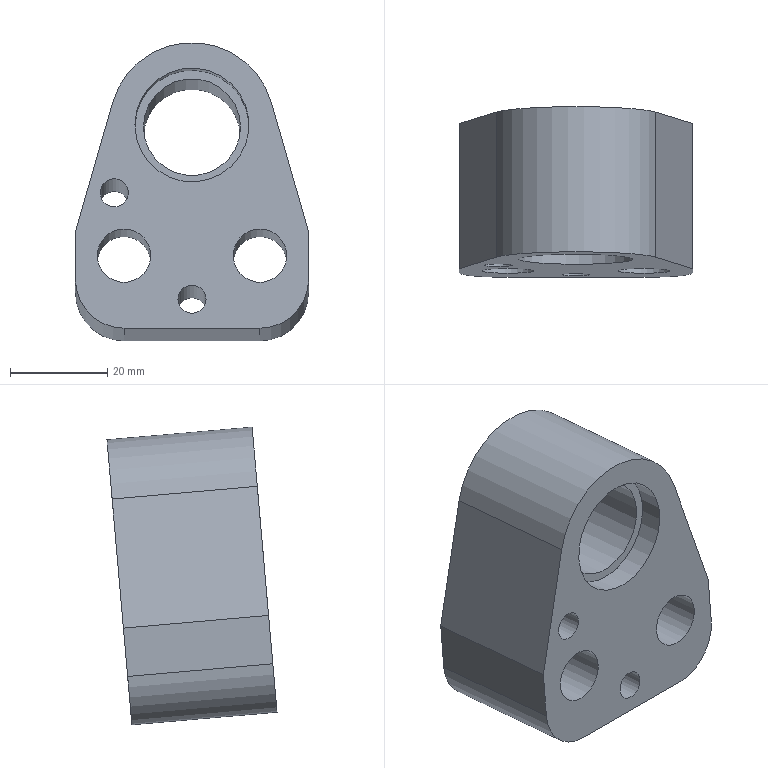Part | NX | features CP-AP 20 2 | 1 solid | 21 faces | box 48 x 35.028 x 61.39 mm | volume 48233 mm3 | cylinder 11 | plane 10 | commonest cylinder face diameters 20 x3 5.8 x2 11 x2 17 x2 23.5 x1 34 x1
STEP:
#1=CARTESIAN_POINT('',(-346.976,-117.842,-64.222));
#2=VERTEX_POINT('',#1);
#3=CARTESIAN_POINT('',(-346.976,-116.971,-54.26));
#4=VERTEX_POINT('',#3);
#5=CARTESIAN_POINT('',(-346.976,-118.714,-74.184));
#6=DIRECTION('',(0.,0.08716,0.9962));
#7=VECTOR('',#6,1000.);
#8=LINE('',#5,#7);
#9=EDGE_CURVE('',#2,#4,#8,.T.);
#10=ORIENTED_EDGE('',*,*,#9,.F.);
#11=CARTESIAN_POINT('',(-346.976,-147.728,-61.607));
#12=VERTEX_POINT('',#11);
#13=CARTESIAN_POINT('',(-346.976,-117.842,-64.222));
#14=DIRECTION('',(0.,-0.9962,0.08716));
#15=VECTOR('',#14,1000.);
#16=LINE('',#13,#15);
#17=EDGE_CURVE('',#2,#12,#16,.T.);
#18=ORIENTED_EDGE('',*,*,#17,.T.);
#19=CARTESIAN_POINT('',(-346.976,-146.856,-51.645));
#20=VERTEX_POINT('',#19);
#21=CARTESIAN_POINT('',(-346.976,-148.6,-71.569));
#22=DIRECTION('',(0.,0.08716,0.9962));
#23=VECTOR('',#22,1000.);
#24=LINE('',#21,#23);
#25=EDGE_CURVE('',#12,#20,#24,.T.);
#26=ORIENTED_EDGE('',*,*,#25,.T.);
#27=CARTESIAN_POINT('',(-346.976,-116.971,-54.26));
#28=DIRECTION('',(0.,-0.9962,0.08716));
#29=VECTOR('',#28,1000.);
#30=LINE('',#27,#29);
#31=EDGE_CURVE('',#4,#20,#30,.T.);
#32=ORIENTED_EDGE('',*,*,#31,.F.);
#33=EDGE_LOOP('',(#10,#18,#26,#32));
#34=FACE_BOUND('',#33,.T.);
#35=CARTESIAN_POINT('',(-346.976,-118.714,-74.184));
#36=DIRECTION('',(1.,0.,0.));
#37=DIRECTION('',(0.,-0.9962,0.08716));
#38=AXIS2_PLACEMENT_3D('',#35,#36,#37);
#39=PLANE('',#38);
#40=ADVANCED_FACE('',(#34),#39,.F.);
#41=CARTESIAN_POINT('',(-339.316,-144.53,-25.058));
#42=VERTEX_POINT('',#41);
#43=CARTESIAN_POINT('',(-346.976,-146.856,-51.645));
#44=DIRECTION('',(0.2759,0.08377,0.9575));
#45=VECTOR('',#44,1000.);
#46=LINE('',#43,#45);
#47=EDGE_CURVE('',#20,#42,#46,.T.);
#48=ORIENTED_EDGE('',*,*,#47,.T.);
#49=CARTESIAN_POINT('',(-339.316,-114.644,-27.672));
#50=VERTEX_POINT('',#49);
#51=CARTESIAN_POINT('',(-339.316,-114.644,-27.672));
#52=DIRECTION('',(0.,-0.9962,0.08716));
#53=VECTOR('',#52,1000.);
#54=LINE('',#51,#53);
#55=EDGE_CURVE('',#50,#42,#54,.T.);
#56=ORIENTED_EDGE('',*,*,#55,.F.);
#57=CARTESIAN_POINT('',(-346.976,-116.971,-54.26));
#58=DIRECTION('',(0.2759,0.08377,0.9575));
#59=VECTOR('',#58,1000.);
#60=LINE('',#57,#59);
#61=EDGE_CURVE('',#4,#50,#60,.T.);
#62=ORIENTED_EDGE('',*,*,#61,.F.);
#63=ORIENTED_EDGE('',*,*,#31,.T.);
#64=EDGE_LOOP('',(#48,#56,#62,#63));
#65=FACE_BOUND('',#64,.T.);
#66=CARTESIAN_POINT('',(-346.976,-116.971,-54.26));
#67=DIRECTION('',(0.9612,-0.02404,-0.2748));
#68=DIRECTION('',(-0.2758,-0.05971,-0.9594));
#69=AXIS2_PLACEMENT_3D('',#66,#67,#68);
#70=PLANE('',#69);
#71=ADVANCED_FACE('',(#65),#70,.F.);
#72=CARTESIAN_POINT('',(-306.636,-144.53,-25.058));
#73=VERTEX_POINT('',#72);
#74=CARTESIAN_POINT('',(-322.976,-144.939,-29.729));
#75=DIRECTION('',(0.,-0.9962,0.08716));
#76=DIRECTION('',(0.,-0.08716,-0.9962));
#77=AXIS2_PLACEMENT_3D('',#74,#75,#76);
#78=CIRCLE('',#77,17.);
#79=EDGE_CURVE('',#73,#42,#78,.T.);
#80=ORIENTED_EDGE('',*,*,#79,.F.);
#81=CARTESIAN_POINT('',(-306.636,-114.644,-27.672));
#82=VERTEX_POINT('',#81);
#83=CARTESIAN_POINT('',(-306.636,-114.644,-27.672));
#84=DIRECTION('',(0.,-0.9962,0.08716));
#85=VECTOR('',#84,1000.);
#86=LINE('',#83,#85);
#87=EDGE_CURVE('',#82,#73,#86,.T.);
#88=ORIENTED_EDGE('',*,*,#87,.F.);
#89=CARTESIAN_POINT('',(-322.976,-115.053,-32.344));
#90=DIRECTION('',(0.,-0.9962,0.08716));
#91=DIRECTION('',(0.,-0.08716,-0.9962));
#92=AXIS2_PLACEMENT_3D('',#89,#90,#91);
#93=CIRCLE('',#92,17.);
#94=EDGE_CURVE('',#82,#50,#93,.T.);
#95=ORIENTED_EDGE('',*,*,#94,.T.);
#96=ORIENTED_EDGE('',*,*,#55,.T.);
#97=EDGE_LOOP('',(#80,#88,#95,#96));
#98=FACE_BOUND('',#97,.T.);
#99=CARTESIAN_POINT('',(-322.976,-115.053,-32.344));
#100=DIRECTION('',(0.,-0.9962,0.08716));
#101=DIRECTION('',(-1.,0.,0.));
#102=AXIS2_PLACEMENT_3D('',#99,#100,#101);
#103=CYLINDRICAL_SURFACE('',#102,17.);
#104=ADVANCED_FACE('',(#98),#103,.T.);
#105=CARTESIAN_POINT('',(-298.976,-146.856,-51.645));
#106=VERTEX_POINT('',#105);
#107=CARTESIAN_POINT('',(-298.976,-146.856,-51.645));
#108=DIRECTION('',(-0.2759,0.08377,0.9575));
#109=VECTOR('',#108,1000.);
#110=LINE('',#107,#109);
#111=EDGE_CURVE('',#106,#73,#110,.T.);
#112=ORIENTED_EDGE('',*,*,#111,.F.);
#113=CARTESIAN_POINT('',(-298.976,-116.971,-54.26));
#114=VERTEX_POINT('',#113);
#115=CARTESIAN_POINT('',(-298.976,-116.971,-54.26));
#116=DIRECTION('',(0.,-0.9962,0.08716));
#117=VECTOR('',#116,1000.);
#118=LINE('',#115,#117);
#119=EDGE_CURVE('',#114,#106,#118,.T.);
#120=ORIENTED_EDGE('',*,*,#119,.F.);
#121=CARTESIAN_POINT('',(-298.976,-116.971,-54.26));
#122=DIRECTION('',(-0.2759,0.08377,0.9575));
#123=VECTOR('',#122,1000.);
#124=LINE('',#121,#123);
#125=EDGE_CURVE('',#114,#82,#124,.T.);
#126=ORIENTED_EDGE('',*,*,#125,.T.);
#127=ORIENTED_EDGE('',*,*,#87,.T.);
#128=EDGE_LOOP('',(#112,#120,#126,#127));
#129=FACE_BOUND('',#128,.T.);
#130=CARTESIAN_POINT('',(-298.976,-116.971,-54.26));
#131=DIRECTION('',(0.9612,0.02404,0.2748));
#132=DIRECTION('',(0.2758,-0.1078,-0.9552));
#133=AXIS2_PLACEMENT_3D('',#130,#131,#132);
#134=PLANE('',#133);
#135=ADVANCED_FACE('',(#129),#134,.T.);
#136=CARTESIAN_POINT('',(-298.976,-147.728,-61.607));
#137=VERTEX_POINT('',#136);
#138=CARTESIAN_POINT('',(-298.976,-148.6,-71.569));
#139=DIRECTION('',(0.,0.08716,0.9962));
#140=VECTOR('',#139,1000.);
#141=LINE('',#138,#140);
#142=EDGE_CURVE('',#137,#106,#141,.T.);
#143=ORIENTED_EDGE('',*,*,#142,.F.);
#144=CARTESIAN_POINT('',(-298.976,-117.842,-64.222));
#145=VERTEX_POINT('',#144);
#146=CARTESIAN_POINT('',(-298.976,-117.842,-64.222));
#147=DIRECTION('',(0.,-0.9962,0.08716));
#148=VECTOR('',#147,1000.);
#149=LINE('',#146,#148);
#150=EDGE_CURVE('',#137,#145,#149,.F.);
#151=ORIENTED_EDGE('',*,*,#150,.T.);
#152=CARTESIAN_POINT('',(-298.976,-118.714,-74.184));
#153=DIRECTION('',(0.,0.08716,0.9962));
#154=VECTOR('',#153,1000.);
#155=LINE('',#152,#154);
#156=EDGE_CURVE('',#145,#114,#155,.T.);
#157=ORIENTED_EDGE('',*,*,#156,.T.);
#158=ORIENTED_EDGE('',*,*,#119,.T.);
#159=EDGE_LOOP('',(#143,#151,#157,#158));
#160=FACE_BOUND('',#159,.T.);
#161=CARTESIAN_POINT('',(-298.976,-118.714,-74.184));
#162=DIRECTION('',(1.,0.,0.));
#163=DIRECTION('',(0.,-0.9962,0.08716));
#164=AXIS2_PLACEMENT_3D('',#161,#162,#163);
#165=PLANE('',#164);
#166=ADVANCED_FACE('',(#160),#165,.T.);
#167=CARTESIAN_POINT('',(-308.976,-148.6,-71.569));
#168=VERTEX_POINT('',#167);
#169=CARTESIAN_POINT('',(-336.976,-148.6,-71.569));
#170=VERTEX_POINT('',#169);
#171=CARTESIAN_POINT('',(-298.976,-148.6,-71.569));
#172=DIRECTION('',(-1.,0.,0.));
#173=VECTOR('',#172,1000.);
#174=LINE('',#171,#173);
#175=EDGE_CURVE('',#168,#170,#174,.T.);
#176=ORIENTED_EDGE('',*,*,#175,.T.);
#177=CARTESIAN_POINT('',(-336.976,-118.714,-74.184));
#178=VERTEX_POINT('',#177);
#179=CARTESIAN_POINT('',(-336.976,-118.714,-74.184));
#180=DIRECTION('',(0.,-0.9962,0.08716));
#181=VECTOR('',#180,1000.);
#182=LINE('',#179,#181);
#183=EDGE_CURVE('',#170,#178,#182,.F.);
#184=ORIENTED_EDGE('',*,*,#183,.T.);
#185=CARTESIAN_POINT('',(-308.976,-118.714,-74.184));
#186=VERTEX_POINT('',#185);
#187=CARTESIAN_POINT('',(-298.976,-118.714,-74.184));
#188=DIRECTION('',(-1.,0.,0.));
#189=VECTOR('',#188,1000.);
#190=LINE('',#187,#189);
#191=EDGE_CURVE('',#186,#178,#190,.T.);
#192=ORIENTED_EDGE('',*,*,#191,.F.);
#193=CARTESIAN_POINT('',(-308.976,-148.6,-71.569));
#194=DIRECTION('',(0.,-0.9962,0.08716));
#195=VECTOR('',#194,1000.);
#196=LINE('',#193,#195);
#197=EDGE_CURVE('',#186,#168,#196,.T.);
#198=ORIENTED_EDGE('',*,*,#197,.T.);
#199=EDGE_LOOP('',(#176,#184,#192,#198));
#200=FACE_BOUND('',#199,.T.);
#201=CARTESIAN_POINT('',(-298.976,-118.714,-74.184));
#202=DIRECTION('',(0.,0.08716,0.9962));
#203=DIRECTION('',(0.9962,-0.08682,0.007596));
#204=AXIS2_PLACEMENT_3D('',#201,#202,#203);
#205=PLANE('',#204);
#206=ADVANCED_FACE('',(#200),#205,.F.);
#207=CARTESIAN_POINT('',(-345.476,-117.406,-59.241));
#208=VERTEX_POINT('',#207);
#209=CARTESIAN_POINT('',(-336.976,-117.406,-59.241));
#210=DIRECTION('',(0.,-0.9962,0.08716));
#211=DIRECTION('',(-1.,0.,0.));
#212=AXIS2_PLACEMENT_3D('',#209,#210,#211);
#213=CIRCLE('',#212,8.5);
#214=EDGE_CURVE('',#208,#208,#213,.T.);
#215=ORIENTED_EDGE('',*,*,#214,.T.);
#216=EDGE_LOOP('',(#215));
#217=FACE_BOUND('',#216,.T.);
#218=CARTESIAN_POINT('',(-317.476,-117.406,-59.241));
#219=VERTEX_POINT('',#218);
#220=CARTESIAN_POINT('',(-308.976,-117.406,-59.241));
#221=DIRECTION('',(0.,-0.9962,0.08716));
#222=DIRECTION('',(-1.,0.,0.));
#223=AXIS2_PLACEMENT_3D('',#220,#221,#222);
#224=CIRCLE('',#223,8.5);
#225=EDGE_CURVE('',#219,#219,#224,.T.);
#226=ORIENTED_EDGE('',*,*,#225,.T.);
#227=EDGE_LOOP('',(#226));
#228=FACE_BOUND('',#227,.T.);
#229=CARTESIAN_POINT('',(-341.876,-116.273,-46.291));
#230=VERTEX_POINT('',#229);
#231=CARTESIAN_POINT('',(-338.976,-116.273,-46.291));
#232=DIRECTION('',(0.,-0.9962,0.08716));
#233=DIRECTION('',(-1.,0.,0.));
#234=AXIS2_PLACEMENT_3D('',#231,#232,#233);
#235=CIRCLE('',#234,2.9);
#236=EDGE_CURVE('',#230,#230,#235,.T.);
#237=ORIENTED_EDGE('',*,*,#236,.T.);
#238=EDGE_LOOP('',(#237));
#239=FACE_BOUND('',#238,.T.);
#240=CARTESIAN_POINT('',(-325.876,-118.191,-68.207));
#241=VERTEX_POINT('',#240);
#242=CARTESIAN_POINT('',(-322.976,-118.191,-68.207));
#243=DIRECTION('',(0.,-0.9962,0.08716));
#244=DIRECTION('',(-1.,0.,0.));
#245=AXIS2_PLACEMENT_3D('',#242,#243,#244);
#246=CIRCLE('',#245,2.9);
#247=EDGE_CURVE('',#241,#241,#246,.T.);
#248=ORIENTED_EDGE('',*,*,#247,.T.);
#249=EDGE_LOOP('',(#248));
#250=FACE_BOUND('',#249,.T.);
#251=CARTESIAN_POINT('',(-332.976,-115.053,-32.344));
#252=VERTEX_POINT('',#251);
#253=CARTESIAN_POINT('',(-322.976,-115.053,-32.344));
#254=DIRECTION('',(0.,-0.9962,0.08716));
#255=DIRECTION('',(-1.,0.,0.));
#256=AXIS2_PLACEMENT_3D('',#253,#254,#255);
#257=CIRCLE('',#256,10.);
#258=EDGE_CURVE('',#252,#252,#257,.T.);
#259=ORIENTED_EDGE('',*,*,#258,.T.);
#260=EDGE_LOOP('',(#259));
#261=FACE_BOUND('',#260,.T.);
#262=ORIENTED_EDGE('',*,*,#191,.T.);
#263=CARTESIAN_POINT('',(-336.976,-117.842,-64.222));
#264=DIRECTION('',(0.,-0.9962,0.08716));
#265=DIRECTION('',(-1.,0.,0.));
#266=AXIS2_PLACEMENT_3D('',#263,#264,#265);
#267=CIRCLE('',#266,10.);
#268=EDGE_CURVE('',#178,#2,#267,.F.);
#269=ORIENTED_EDGE('',*,*,#268,.T.);
#270=ORIENTED_EDGE('',*,*,#9,.T.);
#271=ORIENTED_EDGE('',*,*,#61,.T.);
#272=ORIENTED_EDGE('',*,*,#94,.F.);
#273=ORIENTED_EDGE('',*,*,#125,.F.);
#274=ORIENTED_EDGE('',*,*,#156,.F.);
#275=CARTESIAN_POINT('',(-308.976,-117.842,-64.222));
#276=DIRECTION('',(0.,-0.9962,0.08716));
#277=DIRECTION('',(-1.,0.,0.));
#278=AXIS2_PLACEMENT_3D('',#275,#276,#277);
#279=CIRCLE('',#278,10.);
#280=EDGE_CURVE('',#145,#186,#279,.F.);
#281=ORIENTED_EDGE('',*,*,#280,.T.);
#282=EDGE_LOOP('',(#262,#269,#270,#271,#272,#273,#274,#281));
#283=FACE_BOUND('',#282,.T.);
#284=CARTESIAN_POINT('',(-322.976,-115.053,-32.344));
#285=DIRECTION('',(0.,-0.9962,0.08716));
#286=DIRECTION('',(-1.,0.,0.));
#287=AXIS2_PLACEMENT_3D('',#284,#285,#286);
#288=PLANE('',#287);
#289=ADVANCED_FACE('',(#217,#228,#239,#250,#261,#283),#288,.F.);
#290=CARTESIAN_POINT('',(-342.476,-147.292,-56.626));
#291=VERTEX_POINT('',#290);
#292=CARTESIAN_POINT('',(-336.976,-147.292,-56.626));
#293=DIRECTION('',(0.,-0.9962,0.08716));
#294=DIRECTION('',(-1.,0.,0.));
#295=AXIS2_PLACEMENT_3D('',#292,#293,#294);
#296=CIRCLE('',#295,5.5);
#297=EDGE_CURVE('',#291,#291,#296,.T.);
#298=ORIENTED_EDGE('',*,*,#297,.F.);
#299=EDGE_LOOP('',(#298));
#300=FACE_BOUND('',#299,.T.);
#301=CARTESIAN_POINT('',(-314.476,-147.292,-56.626));
#302=VERTEX_POINT('',#301);
#303=CARTESIAN_POINT('',(-308.976,-147.292,-56.626));
#304=DIRECTION('',(0.,-0.9962,0.08716));
#305=DIRECTION('',(-1.,0.,0.));
#306=AXIS2_PLACEMENT_3D('',#303,#304,#305);
#307=CIRCLE('',#306,5.5);
#308=EDGE_CURVE('',#302,#302,#307,.T.);
#309=ORIENTED_EDGE('',*,*,#308,.F.);
#310=EDGE_LOOP('',(#309));
#311=FACE_BOUND('',#310,.T.);
#312=CARTESIAN_POINT('',(-341.876,-146.159,-43.676));
#313=VERTEX_POINT('',#312);
#314=CARTESIAN_POINT('',(-338.976,-146.159,-43.676));
#315=DIRECTION('',(0.,-0.9962,0.08716));
#316=DIRECTION('',(-1.,0.,0.));
#317=AXIS2_PLACEMENT_3D('',#314,#315,#316);
#318=CIRCLE('',#317,2.9);
#319=EDGE_CURVE('',#313,#313,#318,.T.);
#320=ORIENTED_EDGE('',*,*,#319,.F.);
#321=EDGE_LOOP('',(#320));
#322=FACE_BOUND('',#321,.T.);
#323=CARTESIAN_POINT('',(-325.876,-148.077,-65.592));
#324=VERTEX_POINT('',#323);
#325=CARTESIAN_POINT('',(-322.976,-148.077,-65.592));
#326=DIRECTION('',(0.,-0.9962,0.08716));
#327=DIRECTION('',(-1.,0.,0.));
#328=AXIS2_PLACEMENT_3D('',#325,#326,#327);
#329=CIRCLE('',#328,2.9);
#330=EDGE_CURVE('',#324,#324,#329,.T.);
#331=ORIENTED_EDGE('',*,*,#330,.F.);
#332=EDGE_LOOP('',(#331));
#333=FACE_BOUND('',#332,.T.);
#334=CARTESIAN_POINT('',(-334.726,-144.939,-29.729));
#335=VERTEX_POINT('',#334);
#336=CARTESIAN_POINT('',(-322.976,-144.939,-29.729));
#337=DIRECTION('',(0.,-0.9962,0.08716));
#338=DIRECTION('',(-1.,0.,0.));
#339=AXIS2_PLACEMENT_3D('',#336,#337,#338);
#340=CIRCLE('',#339,11.75);
#341=EDGE_CURVE('',#335,#335,#340,.T.);
#342=ORIENTED_EDGE('',*,*,#341,.F.);
#343=EDGE_LOOP('',(#342));
#344=FACE_BOUND('',#343,.T.);
#345=ORIENTED_EDGE('',*,*,#25,.F.);
#346=CARTESIAN_POINT('',(-336.976,-147.728,-61.607));
#347=DIRECTION('',(0.,-0.9962,0.08716));
#348=DIRECTION('',(-1.,0.,0.));
#349=AXIS2_PLACEMENT_3D('',#346,#347,#348);
#350=CIRCLE('',#349,10.);
#351=EDGE_CURVE('',#12,#170,#350,.T.);
#352=ORIENTED_EDGE('',*,*,#351,.T.);
#353=ORIENTED_EDGE('',*,*,#175,.F.);
#354=CARTESIAN_POINT('',(-308.976,-147.728,-61.607));
#355=DIRECTION('',(0.,-0.9962,0.08716));
#356=DIRECTION('',(-1.,0.,0.));
#357=AXIS2_PLACEMENT_3D('',#354,#355,#356);
#358=CIRCLE('',#357,10.);
#359=EDGE_CURVE('',#168,#137,#358,.T.);
#360=ORIENTED_EDGE('',*,*,#359,.T.);
#361=ORIENTED_EDGE('',*,*,#142,.T.);
#362=ORIENTED_EDGE('',*,*,#111,.T.);
#363=ORIENTED_EDGE('',*,*,#79,.T.);
#364=ORIENTED_EDGE('',*,*,#47,.F.);
#365=EDGE_LOOP('',(#345,#352,#353,#360,#361,#362,#363,#364));
#366=FACE_BOUND('',#365,.T.);
#367=CARTESIAN_POINT('',(-322.976,-144.939,-29.729));
#368=DIRECTION('',(0.,-0.9962,0.08716));
#369=DIRECTION('',(-1.,0.,0.));
#370=AXIS2_PLACEMENT_3D('',#367,#368,#369);
#371=PLANE('',#370);
#372=ADVANCED_FACE('',(#300,#311,#322,#333,#344,#366),#371,.T.);
#373=ORIENTED_EDGE('',*,*,#280,.F.);
#374=ORIENTED_EDGE('',*,*,#150,.F.);
#375=ORIENTED_EDGE('',*,*,#359,.F.);
#376=ORIENTED_EDGE('',*,*,#197,.F.);
#377=EDGE_LOOP('',(#373,#374,#375,#376));
#378=FACE_BOUND('',#377,.T.);
#379=CARTESIAN_POINT('',(-308.976,-117.842,-64.222));
#380=DIRECTION('',(0.,0.9962,-0.08716));
#381=DIRECTION('',(1.,0.,0.));
#382=AXIS2_PLACEMENT_3D('',#379,#380,#381);
#383=CYLINDRICAL_SURFACE('',#382,10.);
#384=ADVANCED_FACE('',(#378),#383,.T.);
#385=ORIENTED_EDGE('',*,*,#268,.F.);
#386=ORIENTED_EDGE('',*,*,#183,.F.);
#387=ORIENTED_EDGE('',*,*,#351,.F.);
#388=ORIENTED_EDGE('',*,*,#17,.F.);
#389=EDGE_LOOP('',(#385,#386,#387,#388));
#390=FACE_BOUND('',#389,.T.);
#391=CARTESIAN_POINT('',(-336.976,-117.842,-64.222));
#392=DIRECTION('',(0.,-0.9962,0.08716));
#393=DIRECTION('',(-1.,0.,0.));
#394=AXIS2_PLACEMENT_3D('',#391,#392,#393);
#395=CYLINDRICAL_SURFACE('',#394,10.);
#396=ADVANCED_FACE('',(#390),#395,.T.);
#397=CARTESIAN_POINT('',(-312.976,-139.958,-30.165));
#398=VERTEX_POINT('',#397);
#399=CARTESIAN_POINT('',(-322.976,-139.958,-30.165));
#400=DIRECTION('',(0.,0.9962,-0.08716));
#401=DIRECTION('',(1.,0.,0.));
#402=AXIS2_PLACEMENT_3D('',#399,#400,#401);
#403=CIRCLE('',#402,10.);
#404=EDGE_CURVE('',#398,#398,#403,.T.);
#405=ORIENTED_EDGE('',*,*,#404,.T.);
#406=EDGE_LOOP('',(#405));
#407=FACE_BOUND('',#406,.T.);
#408=CARTESIAN_POINT('',(-334.726,-139.958,-30.165));
#409=VERTEX_POINT('',#408);
#410=CARTESIAN_POINT('',(-322.976,-139.958,-30.165));
#411=DIRECTION('',(0.,-0.9962,0.08716));
#412=DIRECTION('',(-1.,0.,0.));
#413=AXIS2_PLACEMENT_3D('',#410,#411,#412);
#414=CIRCLE('',#413,11.75);
#415=EDGE_CURVE('',#409,#409,#414,.T.);
#416=ORIENTED_EDGE('',*,*,#415,.T.);
#417=EDGE_LOOP('',(#416));
#418=FACE_BOUND('',#417,.T.);
#419=CARTESIAN_POINT('',(-322.976,-139.958,-30.165));
#420=DIRECTION('',(0.,0.9962,-0.08716));
#421=DIRECTION('',(1.,0.,0.));
#422=AXIS2_PLACEMENT_3D('',#419,#420,#421);
#423=PLANE('',#422);
#424=ADVANCED_FACE('',(#407,#418),#423,.F.);
#425=ORIENTED_EDGE('',*,*,#341,.T.);
#426=EDGE_LOOP('',(#425));
#427=FACE_BOUND('',#426,.T.);
#428=ORIENTED_EDGE('',*,*,#415,.F.);
#429=EDGE_LOOP('',(#428));
#430=FACE_BOUND('',#429,.T.);
#431=CARTESIAN_POINT('',(-322.976,-145.935,-29.642));
#432=DIRECTION('',(0.,0.9962,-0.08716));
#433=DIRECTION('',(1.,0.,0.));
#434=AXIS2_PLACEMENT_3D('',#431,#432,#433);
#435=CYLINDRICAL_SURFACE('',#434,11.75);
#436=ADVANCED_FACE('',(#427,#430),#435,.F.);
#437=ORIENTED_EDGE('',*,*,#404,.F.);
#438=EDGE_LOOP('',(#437));
#439=FACE_BOUND('',#438,.T.);
#440=ORIENTED_EDGE('',*,*,#258,.F.);
#441=EDGE_LOOP('',(#440));
#442=FACE_BOUND('',#441,.T.);
#443=CARTESIAN_POINT('',(-322.976,-145.935,-29.642));
#444=DIRECTION('',(0.,0.9962,-0.08716));
#445=DIRECTION('',(1.,0.,0.));
#446=AXIS2_PLACEMENT_3D('',#443,#444,#445);
#447=CYLINDRICAL_SURFACE('',#446,10.);
#448=ADVANCED_FACE('',(#439,#442),#447,.F.);
#449=ORIENTED_EDGE('',*,*,#330,.T.);
#450=EDGE_LOOP('',(#449));
#451=FACE_BOUND('',#450,.T.);
#452=ORIENTED_EDGE('',*,*,#247,.F.);
#453=EDGE_LOOP('',(#452));
#454=FACE_BOUND('',#453,.T.);
#455=CARTESIAN_POINT('',(-322.976,-149.073,-65.505));
#456=DIRECTION('',(0.,0.9962,-0.08716));
#457=DIRECTION('',(1.,0.,0.));
#458=AXIS2_PLACEMENT_3D('',#455,#456,#457);
#459=CYLINDRICAL_SURFACE('',#458,2.9);
#460=ADVANCED_FACE('',(#451,#454),#459,.F.);
#461=ORIENTED_EDGE('',*,*,#319,.T.);
#462=EDGE_LOOP('',(#461));
#463=FACE_BOUND('',#462,.T.);
#464=ORIENTED_EDGE('',*,*,#236,.F.);
#465=EDGE_LOOP('',(#464));
#466=FACE_BOUND('',#465,.T.);
#467=CARTESIAN_POINT('',(-338.976,-147.155,-43.589));
#468=DIRECTION('',(0.,0.9962,-0.08716));
#469=DIRECTION('',(1.,0.,0.));
#470=AXIS2_PLACEMENT_3D('',#467,#468,#469);
#471=CYLINDRICAL_SURFACE('',#470,2.9);
#472=ADVANCED_FACE('',(#463,#466),#471,.F.);
#473=CARTESIAN_POINT('',(-314.476,-129.361,-58.195));
#474=VERTEX_POINT('',#473);
#475=CARTESIAN_POINT('',(-308.976,-129.361,-58.195));
#476=DIRECTION('',(0.,-0.9962,0.08716));
#477=DIRECTION('',(-1.,0.,0.));
#478=AXIS2_PLACEMENT_3D('',#475,#476,#477);
#479=CIRCLE('',#478,5.5);
#480=EDGE_CURVE('',#474,#474,#479,.F.);
#481=ORIENTED_EDGE('',*,*,#480,.T.);
#482=EDGE_LOOP('',(#481));
#483=FACE_BOUND('',#482,.T.);
#484=ORIENTED_EDGE('',*,*,#308,.T.);
#485=EDGE_LOOP('',(#484));
#486=FACE_BOUND('',#485,.T.);
#487=CARTESIAN_POINT('',(-308.976,-148.288,-56.539));
#488=DIRECTION('',(0.,0.9962,-0.08716));
#489=DIRECTION('',(1.,0.,0.));
#490=AXIS2_PLACEMENT_3D('',#487,#488,#489);
#491=CYLINDRICAL_SURFACE('',#490,5.5);
#492=ADVANCED_FACE('',(#483,#486),#491,.F.);
#493=CARTESIAN_POINT('',(-342.476,-129.361,-58.195));
#494=VERTEX_POINT('',#493);
#495=CARTESIAN_POINT('',(-336.976,-129.361,-58.195));
#496=DIRECTION('',(0.,-0.9962,0.08716));
#497=DIRECTION('',(-1.,0.,0.));
#498=AXIS2_PLACEMENT_3D('',#495,#496,#497);
#499=CIRCLE('',#498,5.5);
#500=EDGE_CURVE('',#494,#494,#499,.F.);
#501=ORIENTED_EDGE('',*,*,#500,.T.);
#502=EDGE_LOOP('',(#501));
#503=FACE_BOUND('',#502,.T.);
#504=ORIENTED_EDGE('',*,*,#297,.T.);
#505=EDGE_LOOP('',(#504));
#506=FACE_BOUND('',#505,.T.);
#507=CARTESIAN_POINT('',(-336.976,-148.288,-56.539));
#508=DIRECTION('',(0.,0.9962,-0.08716));
#509=DIRECTION('',(1.,0.,0.));
#510=AXIS2_PLACEMENT_3D('',#507,#508,#509);
#511=CYLINDRICAL_SURFACE('',#510,5.5);
#512=ADVANCED_FACE('',(#503,#506),#511,.F.);
#513=CARTESIAN_POINT('',(-300.476,-129.361,-58.195));
#514=VERTEX_POINT('',#513);
#515=CARTESIAN_POINT('',(-308.976,-129.361,-58.195));
#516=DIRECTION('',(0.,0.9962,-0.08716));
#517=DIRECTION('',(1.,0.,0.));
#518=AXIS2_PLACEMENT_3D('',#515,#516,#517);
#519=CIRCLE('',#518,8.5);
#520=EDGE_CURVE('',#514,#514,#519,.T.);
#521=ORIENTED_EDGE('',*,*,#520,.F.);
#522=EDGE_LOOP('',(#521));
#523=FACE_BOUND('',#522,.T.);
#524=ORIENTED_EDGE('',*,*,#225,.F.);
#525=EDGE_LOOP('',(#524));
#526=FACE_BOUND('',#525,.T.);
#527=CARTESIAN_POINT('',(-308.976,-129.361,-58.195));
#528=DIRECTION('',(0.,0.9962,-0.08716));
#529=DIRECTION('',(1.,0.,0.));
#530=AXIS2_PLACEMENT_3D('',#527,#528,#529);
#531=CYLINDRICAL_SURFACE('',#530,8.5);
#532=ADVANCED_FACE('',(#523,#526),#531,.F.);
#533=ORIENTED_EDGE('',*,*,#520,.T.);
#534=EDGE_LOOP('',(#533));
#535=FACE_BOUND('',#534,.T.);
#536=ORIENTED_EDGE('',*,*,#480,.F.);
#537=EDGE_LOOP('',(#536));
#538=FACE_BOUND('',#537,.T.);
#539=CARTESIAN_POINT('',(-308.976,-129.361,-58.195));
#540=DIRECTION('',(0.,-0.9962,0.08716));
#541=DIRECTION('',(-1.,0.,0.));
#542=AXIS2_PLACEMENT_3D('',#539,#540,#541);
#543=PLANE('',#542);
#544=ADVANCED_FACE('',(#535,#538),#543,.F.);
#545=CARTESIAN_POINT('',(-328.476,-129.361,-58.195));
#546=VERTEX_POINT('',#545);
#547=CARTESIAN_POINT('',(-336.976,-129.361,-58.195));
#548=DIRECTION('',(0.,0.9962,-0.08716));
#549=DIRECTION('',(1.,0.,0.));
#550=AXIS2_PLACEMENT_3D('',#547,#548,#549);
#551=CIRCLE('',#550,8.5);
#552=EDGE_CURVE('',#546,#546,#551,.T.);
#553=ORIENTED_EDGE('',*,*,#552,.F.);
#554=EDGE_LOOP('',(#553));
#555=FACE_BOUND('',#554,.T.);
#556=ORIENTED_EDGE('',*,*,#214,.F.);
#557=EDGE_LOOP('',(#556));
#558=FACE_BOUND('',#557,.T.);
#559=CARTESIAN_POINT('',(-336.976,-129.361,-58.195));
#560=DIRECTION('',(0.,0.9962,-0.08716));
#561=DIRECTION('',(1.,0.,0.));
#562=AXIS2_PLACEMENT_3D('',#559,#560,#561);
#563=CYLINDRICAL_SURFACE('',#562,8.5);
#564=ADVANCED_FACE('',(#555,#558),#563,.F.);
#565=ORIENTED_EDGE('',*,*,#552,.T.);
#566=EDGE_LOOP('',(#565));
#567=FACE_BOUND('',#566,.T.);
#568=ORIENTED_EDGE('',*,*,#500,.F.);
#569=EDGE_LOOP('',(#568));
#570=FACE_BOUND('',#569,.T.);
#571=CARTESIAN_POINT('',(-336.976,-129.361,-58.195));
#572=DIRECTION('',(0.,-0.9962,0.08716));
#573=DIRECTION('',(-1.,0.,0.));
#574=AXIS2_PLACEMENT_3D('',#571,#572,#573);
#575=PLANE('',#574);
#576=ADVANCED_FACE('',(#567,#570),#575,.F.);
#577=CLOSED_SHELL('',(#40,#71,#104,#135,#166,#206,#289,#372,#384,#396,#424,#436,#448,#460,#472,#492,#512,#532,#544,#564,#576));
#578=MANIFOLD_SOLID_BREP('',#577);
#579=(LENGTH_UNIT()NAMED_UNIT(*)SI_UNIT(.MILLI.,.METRE.));
#580=UNCERTAINTY_MEASURE_WITH_UNIT(LENGTH_MEASURE(0.00001),#579,'','');
#581=(NAMED_UNIT(*)PLANE_ANGLE_UNIT()SI_UNIT($,.RADIAN.));
#582=(NAMED_UNIT(*)SI_UNIT($,.STERADIAN.)SOLID_ANGLE_UNIT());
#583=(GEOMETRIC_REPRESENTATION_CONTEXT(3)GLOBAL_UNCERTAINTY_ASSIGNED_CONTEXT((#580))GLOBAL_UNIT_ASSIGNED_CONTEXT((#579,#581,#582))REPRESENTATION_CONTEXT('',''));
#584=ADVANCED_BREP_SHAPE_REPRESENTATION('',(#578),#583);